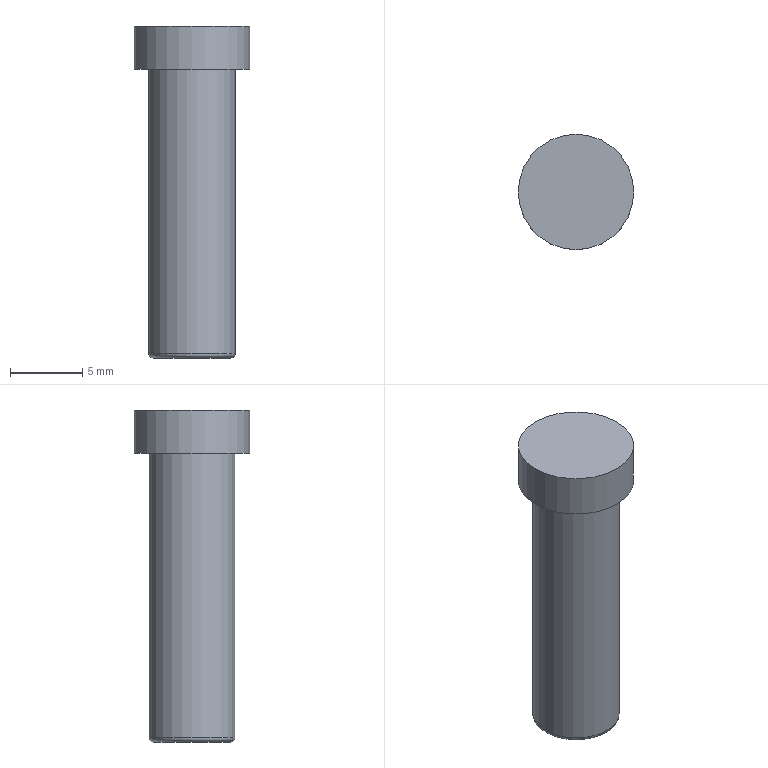Part | STEP file | lll_id2230_x_t | 1 solid | 6 faces | box 8 x 8 x 23 mm | volume 715.927 mm3 | plane 3 | cylinder 2 | torus 1 | commonest cylinder face diameters 6 x1 8 x1
STEP:
#1=CARTESIAN_POINT('',(2468.614,328.696,-13.771));
#2=VERTEX_POINT('',#1);
#3=CARTESIAN_POINT('',(2472.614,328.696,-13.771));
#4=DIRECTION('',(0.,0.,-1.));
#5=DIRECTION('',(-1.,0.,0.));
#6=AXIS2_PLACEMENT_3D('',#3,#4,#5);
#7=CIRCLE('',#6,4.);
#8=EDGE_CURVE('',#2,#2,#7,.T.);
#9=ORIENTED_EDGE('',*,*,#8,.F.);
#10=EDGE_LOOP('',(#9));
#11=FACE_OUTER_BOUND('',#10,.T.);
#12=CARTESIAN_POINT('',(2472.614,328.696,-13.771));
#13=DIRECTION('',(0.,0.,1.));
#14=DIRECTION('',(-1.,0.,0.));
#15=AXIS2_PLACEMENT_3D('',#12,#13,#14);
#16=PLANE('',#15);
#17=ADVANCED_FACE('',(#11),#16,.T.);
#18=CARTESIAN_POINT('',(2475.614,328.696,-16.771));
#19=VERTEX_POINT('',#18);
#20=CARTESIAN_POINT('',(2472.614,328.696,-16.771));
#21=DIRECTION('',(0.,0.,-1.));
#22=DIRECTION('',(1.,0.,0.));
#23=AXIS2_PLACEMENT_3D('',#20,#21,#22);
#24=CIRCLE('',#23,3.);
#25=EDGE_CURVE('',#19,#19,#24,.T.);
#26=ORIENTED_EDGE('',*,*,#25,.F.);
#27=EDGE_LOOP('',(#26));
#28=FACE_BOUND('',#27,.T.);
#29=CARTESIAN_POINT('',(2476.614,328.696,-16.771));
#30=VERTEX_POINT('',#29);
#31=CARTESIAN_POINT('',(2472.614,328.696,-16.771));
#32=DIRECTION('',(0.,0.,1.));
#33=DIRECTION('',(1.,0.,0.));
#34=AXIS2_PLACEMENT_3D('',#31,#32,#33);
#35=CIRCLE('',#34,4.);
#36=EDGE_CURVE('',#30,#30,#35,.T.);
#37=ORIENTED_EDGE('',*,*,#36,.F.);
#38=EDGE_LOOP('',(#37));
#39=FACE_BOUND('',#38,.T.);
#40=CARTESIAN_POINT('',(2472.614,328.696,-16.771));
#41=DIRECTION('',(0.,0.,-1.));
#42=DIRECTION('',(1.,0.,0.));
#43=AXIS2_PLACEMENT_3D('',#40,#41,#42);
#44=PLANE('',#43);
#45=ADVANCED_FACE('',(#28,#39),#44,.T.);
#46=ORIENTED_EDGE('',*,*,#36,.T.);
#47=EDGE_LOOP('',(#46));
#48=FACE_BOUND('',#47,.T.);
#49=ORIENTED_EDGE('',*,*,#8,.T.);
#50=EDGE_LOOP('',(#49));
#51=FACE_BOUND('',#50,.T.);
#52=CARTESIAN_POINT('',(2472.614,328.696,-13.771));
#53=DIRECTION('',(0.,0.,-1.));
#54=DIRECTION('',(1.,0.,0.));
#55=AXIS2_PLACEMENT_3D('',#52,#53,#54);
#56=CYLINDRICAL_SURFACE('',#55,4.);
#57=ADVANCED_FACE('',(#48,#51),#56,.T.);
#58=CARTESIAN_POINT('',(2475.314,328.696,-36.771));
#59=VERTEX_POINT('',#58);
#60=CARTESIAN_POINT('',(2472.614,328.696,-36.771));
#61=DIRECTION('',(0.,0.,-1.));
#62=DIRECTION('',(1.,0.,0.));
#63=AXIS2_PLACEMENT_3D('',#60,#61,#62);
#64=CIRCLE('',#63,2.7);
#65=EDGE_CURVE('',#59,#59,#64,.T.);
#66=ORIENTED_EDGE('',*,*,#65,.T.);
#67=EDGE_LOOP('',(#66));
#68=FACE_OUTER_BOUND('',#67,.T.);
#69=CARTESIAN_POINT('',(2472.614,328.696,-36.771));
#70=DIRECTION('',(0.,0.,-1.));
#71=DIRECTION('',(1.,0.,0.));
#72=AXIS2_PLACEMENT_3D('',#69,#70,#71);
#73=PLANE('',#72);
#74=ADVANCED_FACE('',(#68),#73,.T.);
#75=CARTESIAN_POINT('',(2475.614,328.696,-36.471));
#76=VERTEX_POINT('',#75);
#77=CARTESIAN_POINT('',(2472.614,328.696,-36.471));
#78=DIRECTION('',(0.,0.,1.));
#79=DIRECTION('',(1.,0.,0.));
#80=AXIS2_PLACEMENT_3D('',#77,#78,#79);
#81=CIRCLE('',#80,3.);
#82=EDGE_CURVE('',#76,#76,#81,.T.);
#83=ORIENTED_EDGE('',*,*,#82,.T.);
#84=EDGE_LOOP('',(#83));
#85=FACE_BOUND('',#84,.T.);
#86=ORIENTED_EDGE('',*,*,#25,.T.);
#87=EDGE_LOOP('',(#86));
#88=FACE_BOUND('',#87,.T.);
#89=CARTESIAN_POINT('',(2472.614,328.696,23.229));
#90=DIRECTION('',(0.,0.,-1.));
#91=DIRECTION('',(1.,0.,0.));
#92=AXIS2_PLACEMENT_3D('',#89,#90,#91);
#93=CYLINDRICAL_SURFACE('',#92,3.);
#94=ADVANCED_FACE('',(#85,#88),#93,.T.);
#95=ORIENTED_EDGE('',*,*,#65,.F.);
#96=EDGE_LOOP('',(#95));
#97=FACE_BOUND('',#96,.T.);
#98=ORIENTED_EDGE('',*,*,#82,.F.);
#99=EDGE_LOOP('',(#98));
#100=FACE_BOUND('',#99,.T.);
#101=CARTESIAN_POINT('',(2472.614,328.696,-36.471));
#102=DIRECTION('',(0.,0.,-1.));
#103=DIRECTION('',(1.,0.,0.));
#104=AXIS2_PLACEMENT_3D('',#101,#102,#103);
#105=TOROIDAL_SURFACE('',#104,2.7,0.3);
#106=ADVANCED_FACE('',(#97,#100),#105,.T.);
#107=CLOSED_SHELL('',(#17,#45,#57,#74,#94,#106));
#108=MANIFOLD_SOLID_BREP('',#107);
#109=(LENGTH_UNIT()NAMED_UNIT(*)SI_UNIT(.MILLI.,.METRE.));
#110=UNCERTAINTY_MEASURE_WITH_UNIT(LENGTH_MEASURE(0.00002),#109,'','');
#111=(NAMED_UNIT(*)PLANE_ANGLE_UNIT()SI_UNIT($,.RADIAN.));
#112=PLANE_ANGLE_MEASURE_WITH_UNIT(PLANE_ANGLE_MEASURE(0.01745),#111);
#113=DIMENSIONAL_EXPONENTS(0.,0.,0.,0.,0.,0.,0.);
#114=(CONVERSION_BASED_UNIT('DEGREE',#112)NAMED_UNIT(#113)PLANE_ANGLE_UNIT());
#115=(NAMED_UNIT(*)SI_UNIT($,.STERADIAN.)SOLID_ANGLE_UNIT());
#116=(GEOMETRIC_REPRESENTATION_CONTEXT(3)GLOBAL_UNCERTAINTY_ASSIGNED_CONTEXT((#110))GLOBAL_UNIT_ASSIGNED_CONTEXT((#109,#114,#115))REPRESENTATION_CONTEXT('',''));
#117=ADVANCED_BREP_SHAPE_REPRESENTATION('',(#108),#116);